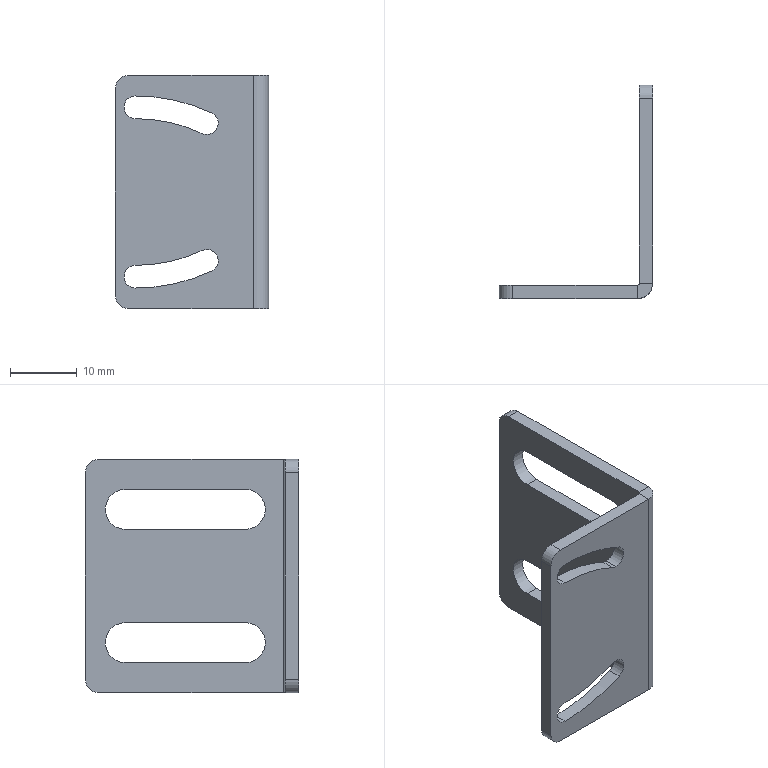Part | SolidWorks | features ICE 2, Fillet 1, FlatPattern 1, HoleWzd 1, MirrorPattern 1, SMBaseFlange 1, SheetMetal 1 | 1 solid | 35 faces | box 23 x 32 x 35 mm | volume 2932 mm3 | cylinder 19 | plane 16 | commonest cylinder face diameters 3.4 x5 4 x4 6 x4 47.4 x2 54.2 x2 0.6 x1
STEP:
#1=CARTESIAN_POINT('',(13.735,0.,26.12));
#2=VERTEX_POINT('',#1);
#3=CARTESIAN_POINT('',(14.453,0.,29.361));
#4=VERTEX_POINT('',#3);
#5=CARTESIAN_POINT('',(13.735,0.,27.82));
#6=DIRECTION('',(0.,-1.,0.));
#7=DIRECTION('',(0.,0.,1.));
#8=AXIS2_PLACEMENT_3D('',#5,#6,#7);
#9=CIRCLE('',#8,1.7);
#10=EDGE_CURVE('',#2,#4,#9,.T.);
#11=ORIENTED_EDGE('',*,*,#10,.F.);
#12=CARTESIAN_POINT('',(13.735,-2.,26.12));
#13=VERTEX_POINT('',#12);
#14=CARTESIAN_POINT('',(13.735,30.,26.12));
#15=DIRECTION('',(0.,-1.,0.));
#16=VECTOR('',#15,1000.);
#17=LINE('',#14,#16);
#18=EDGE_CURVE('',#2,#13,#17,.T.);
#19=ORIENTED_EDGE('',*,*,#18,.T.);
#20=CARTESIAN_POINT('',(14.453,-2.,29.361));
#21=VERTEX_POINT('',#20);
#22=CARTESIAN_POINT('',(13.735,-2.,27.82));
#23=DIRECTION('',(0.,1.,0.));
#24=DIRECTION('',(0.,0.,1.));
#25=AXIS2_PLACEMENT_3D('',#22,#23,#24);
#26=CIRCLE('',#25,1.7);
#27=EDGE_CURVE('',#21,#13,#26,.T.);
#28=ORIENTED_EDGE('',*,*,#27,.F.);
#29=CARTESIAN_POINT('',(14.453,30.,29.361));
#30=DIRECTION('',(0.,-1.,0.));
#31=VECTOR('',#30,1000.);
#32=LINE('',#29,#31);
#33=EDGE_CURVE('',#4,#21,#32,.T.);
#34=ORIENTED_EDGE('',*,*,#33,.F.);
#35=EDGE_LOOP('',(#11,#19,#28,#34));
#36=FACE_OUTER_BOUND('',#35,.T.);
#37=CARTESIAN_POINT('',(13.735,30.,27.82));
#38=DIRECTION('',(0.,-1.,0.));
#39=DIRECTION('',(0.,0.,-1.));
#40=AXIS2_PLACEMENT_3D('',#37,#38,#39);
#41=CYLINDRICAL_SURFACE('',#40,1.7);
#42=ADVANCED_FACE('',(#36),#41,.F.);
#43=CARTESIAN_POINT('',(3.,0.,6.5));
#44=VERTEX_POINT('',#43);
#45=CARTESIAN_POINT('',(13.016,0.,8.721));
#46=VERTEX_POINT('',#45);
#47=CARTESIAN_POINT('',(3.,0.,30.2));
#48=DIRECTION('',(0.,-1.,0.));
#49=DIRECTION('',(0.,0.,1.));
#50=AXIS2_PLACEMENT_3D('',#47,#48,#49);
#51=CIRCLE('',#50,23.7);
#52=EDGE_CURVE('',#44,#46,#51,.T.);
#53=ORIENTED_EDGE('',*,*,#52,.F.);
#54=CARTESIAN_POINT('',(3.,0.,3.1));
#55=VERTEX_POINT('',#54);
#56=CARTESIAN_POINT('',(3.,0.,4.8));
#57=DIRECTION('',(0.,1.,0.));
#58=DIRECTION('',(0.,0.,1.));
#59=AXIS2_PLACEMENT_3D('',#56,#57,#58);
#60=CIRCLE('',#59,1.7);
#61=EDGE_CURVE('',#55,#44,#60,.T.);
#62=ORIENTED_EDGE('',*,*,#61,.F.);
#63=CARTESIAN_POINT('',(14.453,0.,5.639));
#64=VERTEX_POINT('',#63);
#65=CARTESIAN_POINT('',(3.,0.,30.2));
#66=DIRECTION('',(0.,1.,0.));
#67=DIRECTION('',(0.,0.,1.));
#68=AXIS2_PLACEMENT_3D('',#65,#66,#67);
#69=CIRCLE('',#68,27.1);
#70=EDGE_CURVE('',#64,#55,#69,.T.);
#71=ORIENTED_EDGE('',*,*,#70,.F.);
#72=CARTESIAN_POINT('',(13.735,0.,7.18));
#73=DIRECTION('',(0.,1.,0.));
#74=DIRECTION('',(0.,0.,1.));
#75=AXIS2_PLACEMENT_3D('',#72,#73,#74);
#76=CIRCLE('',#75,1.7);
#77=EDGE_CURVE('',#46,#64,#76,.T.);
#78=ORIENTED_EDGE('',*,*,#77,.F.);
#79=EDGE_LOOP('',(#53,#62,#71,#78));
#80=FACE_BOUND('',#79,.T.);
#81=CARTESIAN_POINT('',(0.,0.,33.));
#82=VERTEX_POINT('',#81);
#83=CARTESIAN_POINT('',(0.,0.,2.));
#84=VERTEX_POINT('',#83);
#85=CARTESIAN_POINT('',(0.,0.,35.));
#86=DIRECTION('',(0.,0.,-1.));
#87=VECTOR('',#86,1000.);
#88=LINE('',#85,#87);
#89=EDGE_CURVE('',#82,#84,#88,.T.);
#90=ORIENTED_EDGE('',*,*,#89,.F.);
#91=CARTESIAN_POINT('',(2.,0.,35.));
#92=VERTEX_POINT('',#91);
#93=CARTESIAN_POINT('',(2.,0.,33.));
#94=DIRECTION('',(0.,1.,0.));
#95=DIRECTION('',(0.,0.,1.));
#96=AXIS2_PLACEMENT_3D('',#93,#94,#95);
#97=CIRCLE('',#96,2.);
#98=EDGE_CURVE('',#82,#92,#97,.T.);
#99=ORIENTED_EDGE('',*,*,#98,.T.);
#100=CARTESIAN_POINT('',(20.7,0.,35.));
#101=VERTEX_POINT('',#100);
#102=CARTESIAN_POINT('',(0.,0.,35.));
#103=DIRECTION('',(1.,0.,0.));
#104=VECTOR('',#103,1000.);
#105=LINE('',#102,#104);
#106=EDGE_CURVE('',#92,#101,#105,.T.);
#107=ORIENTED_EDGE('',*,*,#106,.T.);
#108=CARTESIAN_POINT('',(20.7,0.,0.));
#109=VERTEX_POINT('',#108);
#110=CARTESIAN_POINT('',(20.7,0.,35.));
#111=DIRECTION('',(0.,0.,-1.));
#112=VECTOR('',#111,1000.);
#113=LINE('',#110,#112);
#114=EDGE_CURVE('',#101,#109,#113,.T.);
#115=ORIENTED_EDGE('',*,*,#114,.T.);
#116=CARTESIAN_POINT('',(2.,0.,0.));
#117=VERTEX_POINT('',#116);
#118=CARTESIAN_POINT('',(0.,0.,0.));
#119=DIRECTION('',(1.,0.,0.));
#120=VECTOR('',#119,1000.);
#121=LINE('',#118,#120);
#122=EDGE_CURVE('',#117,#109,#121,.T.);
#123=ORIENTED_EDGE('',*,*,#122,.F.);
#124=CARTESIAN_POINT('',(2.,0.,2.));
#125=DIRECTION('',(0.,1.,0.));
#126=DIRECTION('',(0.,0.,1.));
#127=AXIS2_PLACEMENT_3D('',#124,#125,#126);
#128=CIRCLE('',#127,2.);
#129=EDGE_CURVE('',#117,#84,#128,.T.);
#130=ORIENTED_EDGE('',*,*,#129,.T.);
#131=EDGE_LOOP('',(#90,#99,#107,#115,#123,#130));
#132=FACE_OUTER_BOUND('',#131,.T.);
#133=CARTESIAN_POINT('',(13.016,0.,26.279));
#134=VERTEX_POINT('',#133);
#135=CARTESIAN_POINT('',(13.735,0.,27.82));
#136=DIRECTION('',(0.,-1.,0.));
#137=DIRECTION('',(0.,0.,1.));
#138=AXIS2_PLACEMENT_3D('',#135,#136,#137);
#139=CIRCLE('',#138,1.7);
#140=EDGE_CURVE('',#134,#2,#139,.T.);
#141=ORIENTED_EDGE('',*,*,#140,.T.);
#142=ORIENTED_EDGE('',*,*,#10,.T.);
#143=CARTESIAN_POINT('',(3.,0.,31.9));
#144=VERTEX_POINT('',#143);
#145=CARTESIAN_POINT('',(3.,0.,4.8));
#146=DIRECTION('',(0.,-1.,0.));
#147=DIRECTION('',(0.,0.,1.));
#148=AXIS2_PLACEMENT_3D('',#145,#146,#147);
#149=CIRCLE('',#148,27.1);
#150=EDGE_CURVE('',#4,#144,#149,.T.);
#151=ORIENTED_EDGE('',*,*,#150,.T.);
#152=CARTESIAN_POINT('',(3.,0.,28.5));
#153=VERTEX_POINT('',#152);
#154=CARTESIAN_POINT('',(3.,0.,30.2));
#155=DIRECTION('',(0.,1.,0.));
#156=DIRECTION('',(0.,0.,1.));
#157=AXIS2_PLACEMENT_3D('',#154,#155,#156);
#158=CIRCLE('',#157,1.7);
#159=EDGE_CURVE('',#153,#144,#158,.T.);
#160=ORIENTED_EDGE('',*,*,#159,.F.);
#161=CARTESIAN_POINT('',(3.,0.,4.8));
#162=DIRECTION('',(0.,1.,0.));
#163=DIRECTION('',(0.,0.,1.));
#164=AXIS2_PLACEMENT_3D('',#161,#162,#163);
#165=CIRCLE('',#164,23.7);
#166=EDGE_CURVE('',#153,#134,#165,.T.);
#167=ORIENTED_EDGE('',*,*,#166,.T.);
#168=EDGE_LOOP('',(#141,#142,#151,#160,#167));
#169=FACE_BOUND('',#168,.T.);
#170=CARTESIAN_POINT('',(0.,0.,35.));
#171=DIRECTION('',(0.,1.,0.));
#172=DIRECTION('',(0.,0.,1.));
#173=AXIS2_PLACEMENT_3D('',#170,#171,#172);
#174=PLANE('',#173);
#175=ADVANCED_FACE('',(#80,#132,#169),#174,.T.);
#176=CARTESIAN_POINT('',(2.,-2.,35.));
#177=VERTEX_POINT('',#176);
#178=CARTESIAN_POINT('',(20.7,-2.,35.));
#179=VERTEX_POINT('',#178);
#180=CARTESIAN_POINT('',(0.,-2.,35.));
#181=DIRECTION('',(1.,0.,0.));
#182=VECTOR('',#181,1000.);
#183=LINE('',#180,#182);
#184=EDGE_CURVE('',#177,#179,#183,.T.);
#185=ORIENTED_EDGE('',*,*,#184,.F.);
#186=CARTESIAN_POINT('',(0.,-2.,33.));
#187=VERTEX_POINT('',#186);
#188=CARTESIAN_POINT('',(2.,-2.,33.));
#189=DIRECTION('',(0.,-1.,0.));
#190=DIRECTION('',(0.,0.,1.));
#191=AXIS2_PLACEMENT_3D('',#188,#189,#190);
#192=CIRCLE('',#191,2.);
#193=EDGE_CURVE('',#177,#187,#192,.T.);
#194=ORIENTED_EDGE('',*,*,#193,.T.);
#195=CARTESIAN_POINT('',(0.,-2.,2.));
#196=VERTEX_POINT('',#195);
#197=CARTESIAN_POINT('',(0.,-2.,35.));
#198=DIRECTION('',(0.,0.,-1.));
#199=VECTOR('',#198,1000.);
#200=LINE('',#197,#199);
#201=EDGE_CURVE('',#187,#196,#200,.T.);
#202=ORIENTED_EDGE('',*,*,#201,.T.);
#203=CARTESIAN_POINT('',(2.,-2.,0.));
#204=VERTEX_POINT('',#203);
#205=CARTESIAN_POINT('',(2.,-2.,2.));
#206=DIRECTION('',(0.,-1.,0.));
#207=DIRECTION('',(0.,0.,1.));
#208=AXIS2_PLACEMENT_3D('',#205,#206,#207);
#209=CIRCLE('',#208,2.);
#210=EDGE_CURVE('',#196,#204,#209,.T.);
#211=ORIENTED_EDGE('',*,*,#210,.T.);
#212=CARTESIAN_POINT('',(20.7,-2.,0.));
#213=VERTEX_POINT('',#212);
#214=CARTESIAN_POINT('',(0.,-2.,0.));
#215=DIRECTION('',(1.,0.,0.));
#216=VECTOR('',#215,1000.);
#217=LINE('',#214,#216);
#218=EDGE_CURVE('',#204,#213,#217,.T.);
#219=ORIENTED_EDGE('',*,*,#218,.T.);
#220=CARTESIAN_POINT('',(20.7,-2.,35.));
#221=DIRECTION('',(0.,0.,-1.));
#222=VECTOR('',#221,1000.);
#223=LINE('',#220,#222);
#224=EDGE_CURVE('',#179,#213,#223,.T.);
#225=ORIENTED_EDGE('',*,*,#224,.F.);
#226=EDGE_LOOP('',(#185,#194,#202,#211,#219,#225));
#227=FACE_OUTER_BOUND('',#226,.T.);
#228=CARTESIAN_POINT('',(3.,-2.,3.1));
#229=VERTEX_POINT('',#228);
#230=CARTESIAN_POINT('',(3.,-2.,6.5));
#231=VERTEX_POINT('',#230);
#232=CARTESIAN_POINT('',(3.,-2.,4.8));
#233=DIRECTION('',(0.,1.,0.));
#234=DIRECTION('',(0.,0.,1.));
#235=AXIS2_PLACEMENT_3D('',#232,#233,#234);
#236=CIRCLE('',#235,1.7);
#237=EDGE_CURVE('',#229,#231,#236,.T.);
#238=ORIENTED_EDGE('',*,*,#237,.T.);
#239=CARTESIAN_POINT('',(13.016,-2.,8.721));
#240=VERTEX_POINT('',#239);
#241=CARTESIAN_POINT('',(3.,-2.,30.2));
#242=DIRECTION('',(0.,1.,0.));
#243=DIRECTION('',(0.,0.,-1.));
#244=AXIS2_PLACEMENT_3D('',#241,#242,#243);
#245=CIRCLE('',#244,23.7);
#246=EDGE_CURVE('',#240,#231,#245,.T.);
#247=ORIENTED_EDGE('',*,*,#246,.F.);
#248=CARTESIAN_POINT('',(14.453,-2.,5.639));
#249=VERTEX_POINT('',#248);
#250=CARTESIAN_POINT('',(13.735,-2.,7.18));
#251=DIRECTION('',(0.,-1.,0.));
#252=DIRECTION('',(0.,0.,-1.));
#253=AXIS2_PLACEMENT_3D('',#250,#251,#252);
#254=CIRCLE('',#253,1.7);
#255=EDGE_CURVE('',#249,#240,#254,.T.);
#256=ORIENTED_EDGE('',*,*,#255,.F.);
#257=CARTESIAN_POINT('',(3.,-2.,30.2));
#258=DIRECTION('',(0.,-1.,0.));
#259=DIRECTION('',(0.,0.,-1.));
#260=AXIS2_PLACEMENT_3D('',#257,#258,#259);
#261=CIRCLE('',#260,27.1);
#262=EDGE_CURVE('',#229,#249,#261,.T.);
#263=ORIENTED_EDGE('',*,*,#262,.F.);
#264=EDGE_LOOP('',(#238,#247,#256,#263));
#265=FACE_BOUND('',#264,.T.);
#266=CARTESIAN_POINT('',(3.,-2.,31.9));
#267=VERTEX_POINT('',#266);
#268=CARTESIAN_POINT('',(3.,-2.,4.8));
#269=DIRECTION('',(0.,1.,0.));
#270=DIRECTION('',(0.,0.,1.));
#271=AXIS2_PLACEMENT_3D('',#268,#269,#270);
#272=CIRCLE('',#271,27.1);
#273=EDGE_CURVE('',#267,#21,#272,.T.);
#274=ORIENTED_EDGE('',*,*,#273,.T.);
#275=ORIENTED_EDGE('',*,*,#27,.T.);
#276=CARTESIAN_POINT('',(13.016,-2.,26.279));
#277=VERTEX_POINT('',#276);
#278=CARTESIAN_POINT('',(13.735,-2.,27.82));
#279=DIRECTION('',(0.,1.,0.));
#280=DIRECTION('',(0.,0.,1.));
#281=AXIS2_PLACEMENT_3D('',#278,#279,#280);
#282=CIRCLE('',#281,1.7);
#283=EDGE_CURVE('',#13,#277,#282,.T.);
#284=ORIENTED_EDGE('',*,*,#283,.T.);
#285=CARTESIAN_POINT('',(3.,-2.,28.5));
#286=VERTEX_POINT('',#285);
#287=CARTESIAN_POINT('',(3.,-2.,4.8));
#288=DIRECTION('',(0.,-1.,0.));
#289=DIRECTION('',(0.,0.,1.));
#290=AXIS2_PLACEMENT_3D('',#287,#288,#289);
#291=CIRCLE('',#290,23.7);
#292=EDGE_CURVE('',#277,#286,#291,.T.);
#293=ORIENTED_EDGE('',*,*,#292,.T.);
#294=CARTESIAN_POINT('',(3.,-2.,30.2));
#295=DIRECTION('',(0.,1.,0.));
#296=DIRECTION('',(0.,0.,1.));
#297=AXIS2_PLACEMENT_3D('',#294,#295,#296);
#298=CIRCLE('',#297,1.7);
#299=EDGE_CURVE('',#286,#267,#298,.T.);
#300=ORIENTED_EDGE('',*,*,#299,.T.);
#301=EDGE_LOOP('',(#274,#275,#284,#293,#300));
#302=FACE_BOUND('',#301,.T.);
#303=CARTESIAN_POINT('',(0.,-2.,35.));
#304=DIRECTION('',(0.,1.,0.));
#305=DIRECTION('',(0.,0.,1.));
#306=AXIS2_PLACEMENT_3D('',#303,#304,#305);
#307=PLANE('',#306);
#308=ADVANCED_FACE('',(#227,#265,#302),#307,.F.);
#309=CARTESIAN_POINT('',(21.,0.3,35.));
#310=VERTEX_POINT('',#309);
#311=CARTESIAN_POINT('',(23.,0.3,35.));
#312=VERTEX_POINT('',#311);
#313=CARTESIAN_POINT('',(21.,0.3,35.));
#314=DIRECTION('',(1.,0.,0.));
#315=VECTOR('',#314,1000.);
#316=LINE('',#313,#315);
#317=EDGE_CURVE('',#310,#312,#316,.T.);
#318=ORIENTED_EDGE('',*,*,#317,.F.);
#319=CARTESIAN_POINT('',(20.7,0.3,35.));
#320=DIRECTION('',(0.,0.,1.));
#321=DIRECTION('',(-1.,0.,0.));
#322=AXIS2_PLACEMENT_3D('',#319,#320,#321);
#323=CIRCLE('',#322,0.3);
#324=EDGE_CURVE('',#101,#310,#323,.T.);
#325=ORIENTED_EDGE('',*,*,#324,.F.);
#326=CARTESIAN_POINT('',(20.7,-2.,35.));
#327=DIRECTION('',(0.,1.,0.));
#328=VECTOR('',#327,1000.);
#329=LINE('',#326,#328);
#330=EDGE_CURVE('',#179,#101,#329,.T.);
#331=ORIENTED_EDGE('',*,*,#330,.F.);
#332=CARTESIAN_POINT('',(20.7,0.3,35.));
#333=DIRECTION('',(0.,0.,1.));
#334=DIRECTION('',(1.,0.,0.));
#335=AXIS2_PLACEMENT_3D('',#332,#333,#334);
#336=CIRCLE('',#335,2.3);
#337=EDGE_CURVE('',#179,#312,#336,.T.);
#338=ORIENTED_EDGE('',*,*,#337,.T.);
#339=EDGE_LOOP('',(#318,#325,#331,#338));
#340=FACE_OUTER_BOUND('',#339,.T.);
#341=CARTESIAN_POINT('',(21.,0.3,35.));
#342=DIRECTION('',(0.,0.,1.));
#343=DIRECTION('',(1.,0.,0.));
#344=AXIS2_PLACEMENT_3D('',#341,#342,#343);
#345=PLANE('',#344);
#346=ADVANCED_FACE('',(#340),#345,.T.);
#347=CARTESIAN_POINT('',(23.,28.,35.));
#348=VERTEX_POINT('',#347);
#349=CARTESIAN_POINT('',(23.,0.,35.));
#350=DIRECTION('',(0.,1.,0.));
#351=VECTOR('',#350,1000.);
#352=LINE('',#349,#351);
#353=EDGE_CURVE('',#312,#348,#352,.T.);
#354=ORIENTED_EDGE('',*,*,#353,.T.);
#355=CARTESIAN_POINT('',(21.,28.,35.));
#356=VERTEX_POINT('',#355);
#357=CARTESIAN_POINT('',(20.7,28.,35.));
#358=DIRECTION('',(-1.,0.,0.));
#359=VECTOR('',#358,1000.);
#360=LINE('',#357,#359);
#361=EDGE_CURVE('',#348,#356,#360,.T.);
#362=ORIENTED_EDGE('',*,*,#361,.T.);
#363=CARTESIAN_POINT('',(21.,0.,35.));
#364=DIRECTION('',(0.,1.,0.));
#365=VECTOR('',#364,1000.);
#366=LINE('',#363,#365);
#367=EDGE_CURVE('',#310,#356,#366,.T.);
#368=ORIENTED_EDGE('',*,*,#367,.F.);
#369=ORIENTED_EDGE('',*,*,#317,.T.);
#370=EDGE_LOOP('',(#354,#362,#368,#369));
#371=FACE_OUTER_BOUND('',#370,.T.);
#372=CARTESIAN_POINT('',(20.7,-2.,35.));
#373=DIRECTION('',(0.,0.,1.));
#374=DIRECTION('',(1.,0.,0.));
#375=AXIS2_PLACEMENT_3D('',#372,#373,#374);
#376=PLANE('',#375);
#377=ADVANCED_FACE('',(#371),#376,.T.);
#378=CARTESIAN_POINT('',(20.7,0.,0.));
#379=DIRECTION('',(0.,-1.,0.));
#380=VECTOR('',#379,1000.);
#381=LINE('',#378,#380);
#382=EDGE_CURVE('',#109,#213,#381,.T.);
#383=ORIENTED_EDGE('',*,*,#382,.F.);
#384=CARTESIAN_POINT('',(21.,0.3,0.));
#385=VERTEX_POINT('',#384);
#386=CARTESIAN_POINT('',(20.7,0.3,0.));
#387=DIRECTION('',(0.,0.,1.));
#388=DIRECTION('',(-1.,0.,0.));
#389=AXIS2_PLACEMENT_3D('',#386,#387,#388);
#390=CIRCLE('',#389,0.3);
#391=EDGE_CURVE('',#109,#385,#390,.T.);
#392=ORIENTED_EDGE('',*,*,#391,.T.);
#393=CARTESIAN_POINT('',(23.,0.3,0.));
#394=VERTEX_POINT('',#393);
#395=CARTESIAN_POINT('',(23.,0.3,0.));
#396=DIRECTION('',(-1.,0.,0.));
#397=VECTOR('',#396,1000.);
#398=LINE('',#395,#397);
#399=EDGE_CURVE('',#394,#385,#398,.T.);
#400=ORIENTED_EDGE('',*,*,#399,.F.);
#401=CARTESIAN_POINT('',(20.7,0.3,0.));
#402=DIRECTION('',(0.,0.,1.));
#403=DIRECTION('',(1.,0.,0.));
#404=AXIS2_PLACEMENT_3D('',#401,#402,#403);
#405=CIRCLE('',#404,2.3);
#406=EDGE_CURVE('',#213,#394,#405,.T.);
#407=ORIENTED_EDGE('',*,*,#406,.F.);
#408=EDGE_LOOP('',(#383,#392,#400,#407));
#409=FACE_OUTER_BOUND('',#408,.T.);
#410=CARTESIAN_POINT('',(20.7,0.,0.));
#411=DIRECTION('',(0.,0.,-1.));
#412=DIRECTION('',(-1.,0.,0.));
#413=AXIS2_PLACEMENT_3D('',#410,#411,#412);
#414=PLANE('',#413);
#415=ADVANCED_FACE('',(#409),#414,.T.);
#416=ORIENTED_EDGE('',*,*,#218,.F.);
#417=CARTESIAN_POINT('',(2.,0.3,0.));
#418=DIRECTION('',(0.,1.,0.));
#419=VECTOR('',#418,1000.);
#420=LINE('',#417,#419);
#421=EDGE_CURVE('',#204,#117,#420,.T.);
#422=ORIENTED_EDGE('',*,*,#421,.T.);
#423=ORIENTED_EDGE('',*,*,#122,.T.);
#424=ORIENTED_EDGE('',*,*,#382,.T.);
#425=EDGE_LOOP('',(#416,#422,#423,#424));
#426=FACE_OUTER_BOUND('',#425,.T.);
#427=CARTESIAN_POINT('',(23.,0.3,0.));
#428=DIRECTION('',(0.,0.,-1.));
#429=DIRECTION('',(-1.,0.,0.));
#430=AXIS2_PLACEMENT_3D('',#427,#428,#429);
#431=PLANE('',#430);
#432=ADVANCED_FACE('',(#426),#431,.T.);
#433=CARTESIAN_POINT('',(23.,6.,10.5));
#434=VERTEX_POINT('',#433);
#435=CARTESIAN_POINT('',(23.,24.,10.5));
#436=VERTEX_POINT('',#435);
#437=CARTESIAN_POINT('',(23.,24.,10.5));
#438=DIRECTION('',(0.,1.,0.));
#439=VECTOR('',#438,1000.);
#440=LINE('',#437,#439);
#441=EDGE_CURVE('',#434,#436,#440,.T.);
#442=ORIENTED_EDGE('',*,*,#441,.T.);
#443=CARTESIAN_POINT('',(23.,24.,4.5));
#444=VERTEX_POINT('',#443);
#445=CARTESIAN_POINT('',(23.,24.,7.5));
#446=DIRECTION('',(-1.,0.,0.));
#447=DIRECTION('',(0.,0.,1.));
#448=AXIS2_PLACEMENT_3D('',#445,#446,#447);
#449=CIRCLE('',#448,3.);
#450=EDGE_CURVE('',#436,#444,#449,.T.);
#451=ORIENTED_EDGE('',*,*,#450,.T.);
#452=CARTESIAN_POINT('',(23.,6.,4.5));
#453=VERTEX_POINT('',#452);
#454=CARTESIAN_POINT('',(23.,24.,4.5));
#455=DIRECTION('',(0.,-1.,0.));
#456=VECTOR('',#455,1000.);
#457=LINE('',#454,#456);
#458=EDGE_CURVE('',#444,#453,#457,.T.);
#459=ORIENTED_EDGE('',*,*,#458,.T.);
#460=CARTESIAN_POINT('',(23.,6.,7.5));
#461=DIRECTION('',(-1.,0.,0.));
#462=DIRECTION('',(0.,0.,1.));
#463=AXIS2_PLACEMENT_3D('',#460,#461,#462);
#464=CIRCLE('',#463,3.);
#465=EDGE_CURVE('',#453,#434,#464,.T.);
#466=ORIENTED_EDGE('',*,*,#465,.T.);
#467=EDGE_LOOP('',(#442,#451,#459,#466));
#468=FACE_BOUND('',#467,.T.);
#469=CARTESIAN_POINT('',(23.,6.,30.5));
#470=VERTEX_POINT('',#469);
#471=CARTESIAN_POINT('',(23.,24.,30.5));
#472=VERTEX_POINT('',#471);
#473=CARTESIAN_POINT('',(23.,24.,30.5));
#474=DIRECTION('',(0.,1.,0.));
#475=VECTOR('',#474,1000.);
#476=LINE('',#473,#475);
#477=EDGE_CURVE('',#470,#472,#476,.T.);
#478=ORIENTED_EDGE('',*,*,#477,.T.);
#479=CARTESIAN_POINT('',(23.,24.,24.5));
#480=VERTEX_POINT('',#479);
#481=CARTESIAN_POINT('',(23.,24.,27.5));
#482=DIRECTION('',(-1.,0.,0.));
#483=DIRECTION('',(0.,0.,1.));
#484=AXIS2_PLACEMENT_3D('',#481,#482,#483);
#485=CIRCLE('',#484,3.);
#486=EDGE_CURVE('',#472,#480,#485,.T.);
#487=ORIENTED_EDGE('',*,*,#486,.T.);
#488=CARTESIAN_POINT('',(23.,6.,24.5));
#489=VERTEX_POINT('',#488);
#490=CARTESIAN_POINT('',(23.,24.,24.5));
#491=DIRECTION('',(0.,-1.,0.));
#492=VECTOR('',#491,1000.);
#493=LINE('',#490,#492);
#494=EDGE_CURVE('',#480,#489,#493,.T.);
#495=ORIENTED_EDGE('',*,*,#494,.T.);
#496=CARTESIAN_POINT('',(23.,6.,27.5));
#497=DIRECTION('',(-1.,0.,0.));
#498=DIRECTION('',(0.,0.,1.));
#499=AXIS2_PLACEMENT_3D('',#496,#497,#498);
#500=CIRCLE('',#499,3.);
#501=EDGE_CURVE('',#489,#470,#500,.T.);
#502=ORIENTED_EDGE('',*,*,#501,.T.);
#503=EDGE_LOOP('',(#478,#487,#495,#502));
#504=FACE_BOUND('',#503,.T.);
#505=CARTESIAN_POINT('',(23.,28.,0.));
#506=VERTEX_POINT('',#505);
#507=CARTESIAN_POINT('',(23.,0.,0.));
#508=DIRECTION('',(0.,1.,0.));
#509=VECTOR('',#508,1000.);
#510=LINE('',#507,#509);
#511=EDGE_CURVE('',#394,#506,#510,.T.);
#512=ORIENTED_EDGE('',*,*,#511,.T.);
#513=CARTESIAN_POINT('',(23.,30.,2.));
#514=VERTEX_POINT('',#513);
#515=CARTESIAN_POINT('',(23.,28.,2.));
#516=DIRECTION('',(1.,0.,0.));
#517=DIRECTION('',(0.,0.,1.));
#518=AXIS2_PLACEMENT_3D('',#515,#516,#517);
#519=CIRCLE('',#518,2.);
#520=EDGE_CURVE('',#506,#514,#519,.T.);
#521=ORIENTED_EDGE('',*,*,#520,.T.);
#522=CARTESIAN_POINT('',(23.,30.,33.));
#523=VERTEX_POINT('',#522);
#524=CARTESIAN_POINT('',(23.,30.,35.));
#525=DIRECTION('',(0.,0.,-1.));
#526=VECTOR('',#525,1000.);
#527=LINE('',#524,#526);
#528=EDGE_CURVE('',#523,#514,#527,.T.);
#529=ORIENTED_EDGE('',*,*,#528,.F.);
#530=CARTESIAN_POINT('',(23.,28.,33.));
#531=DIRECTION('',(1.,0.,0.));
#532=DIRECTION('',(0.,0.,1.));
#533=AXIS2_PLACEMENT_3D('',#530,#531,#532);
#534=CIRCLE('',#533,2.);
#535=EDGE_CURVE('',#523,#348,#534,.T.);
#536=ORIENTED_EDGE('',*,*,#535,.T.);
#537=ORIENTED_EDGE('',*,*,#353,.F.);
#538=CARTESIAN_POINT('',(23.,0.3,35.));
#539=DIRECTION('',(0.,0.,-1.));
#540=VECTOR('',#539,1000.);
#541=LINE('',#538,#540);
#542=EDGE_CURVE('',#312,#394,#541,.T.);
#543=ORIENTED_EDGE('',*,*,#542,.T.);
#544=EDGE_LOOP('',(#512,#521,#529,#536,#537,#543));
#545=FACE_OUTER_BOUND('',#544,.T.);
#546=CARTESIAN_POINT('',(23.,0.,35.));
#547=DIRECTION('',(-1.,0.,0.));
#548=DIRECTION('',(0.,0.,1.));
#549=AXIS2_PLACEMENT_3D('',#546,#547,#548);
#550=PLANE('',#549);
#551=ADVANCED_FACE('',(#468,#504,#545),#550,.F.);
#552=ORIENTED_EDGE('',*,*,#528,.T.);
#553=CARTESIAN_POINT('',(21.,30.,2.));
#554=VERTEX_POINT('',#553);
#555=CARTESIAN_POINT('',(21.,30.,2.));
#556=DIRECTION('',(-1.,0.,0.));
#557=VECTOR('',#556,1000.);
#558=LINE('',#555,#557);
#559=EDGE_CURVE('',#514,#554,#558,.T.);
#560=ORIENTED_EDGE('',*,*,#559,.T.);
#561=CARTESIAN_POINT('',(21.,30.,33.));
#562=VERTEX_POINT('',#561);
#563=CARTESIAN_POINT('',(21.,30.,35.));
#564=DIRECTION('',(0.,0.,-1.));
#565=VECTOR('',#564,1000.);
#566=LINE('',#563,#565);
#567=EDGE_CURVE('',#562,#554,#566,.T.);
#568=ORIENTED_EDGE('',*,*,#567,.F.);
#569=CARTESIAN_POINT('',(21.,30.,33.));
#570=DIRECTION('',(1.,0.,0.));
#571=VECTOR('',#570,1000.);
#572=LINE('',#569,#571);
#573=EDGE_CURVE('',#562,#523,#572,.T.);
#574=ORIENTED_EDGE('',*,*,#573,.T.);
#575=EDGE_LOOP('',(#552,#560,#568,#574));
#576=FACE_OUTER_BOUND('',#575,.T.);
#577=CARTESIAN_POINT('',(21.,30.,35.));
#578=DIRECTION('',(0.,1.,0.));
#579=DIRECTION('',(0.,0.,1.));
#580=AXIS2_PLACEMENT_3D('',#577,#578,#579);
#581=PLANE('',#580);
#582=ADVANCED_FACE('',(#576),#581,.T.);
#583=CARTESIAN_POINT('',(21.,24.,10.5));
#584=VERTEX_POINT('',#583);
#585=CARTESIAN_POINT('',(21.,24.,4.5));
#586=VERTEX_POINT('',#585);
#587=CARTESIAN_POINT('',(21.,24.,7.5));
#588=DIRECTION('',(-1.,0.,0.));
#589=DIRECTION('',(0.,0.,1.));
#590=AXIS2_PLACEMENT_3D('',#587,#588,#589);
#591=CIRCLE('',#590,3.);
#592=EDGE_CURVE('',#584,#586,#591,.T.);
#593=ORIENTED_EDGE('',*,*,#592,.F.);
#594=CARTESIAN_POINT('',(21.,6.,10.5));
#595=VERTEX_POINT('',#594);
#596=CARTESIAN_POINT('',(21.,24.,10.5));
#597=DIRECTION('',(0.,1.,0.));
#598=VECTOR('',#597,1000.);
#599=LINE('',#596,#598);
#600=EDGE_CURVE('',#595,#584,#599,.T.);
#601=ORIENTED_EDGE('',*,*,#600,.F.);
#602=CARTESIAN_POINT('',(21.,6.,4.5));
#603=VERTEX_POINT('',#602);
#604=CARTESIAN_POINT('',(21.,6.,7.5));
#605=DIRECTION('',(-1.,0.,0.));
#606=DIRECTION('',(0.,0.,1.));
#607=AXIS2_PLACEMENT_3D('',#604,#605,#606);
#608=CIRCLE('',#607,3.);
#609=EDGE_CURVE('',#603,#595,#608,.T.);
#610=ORIENTED_EDGE('',*,*,#609,.F.);
#611=CARTESIAN_POINT('',(21.,24.,4.5));
#612=DIRECTION('',(0.,-1.,0.));
#613=VECTOR('',#612,1000.);
#614=LINE('',#611,#613);
#615=EDGE_CURVE('',#586,#603,#614,.T.);
#616=ORIENTED_EDGE('',*,*,#615,.F.);
#617=EDGE_LOOP('',(#593,#601,#610,#616));
#618=FACE_BOUND('',#617,.T.);
#619=CARTESIAN_POINT('',(21.,24.,30.5));
#620=VERTEX_POINT('',#619);
#621=CARTESIAN_POINT('',(21.,24.,24.5));
#622=VERTEX_POINT('',#621);
#623=CARTESIAN_POINT('',(21.,24.,27.5));
#624=DIRECTION('',(-1.,0.,0.));
#625=DIRECTION('',(0.,0.,1.));
#626=AXIS2_PLACEMENT_3D('',#623,#624,#625);
#627=CIRCLE('',#626,3.);
#628=EDGE_CURVE('',#620,#622,#627,.T.);
#629=ORIENTED_EDGE('',*,*,#628,.F.);
#630=CARTESIAN_POINT('',(21.,6.,30.5));
#631=VERTEX_POINT('',#630);
#632=CARTESIAN_POINT('',(21.,24.,30.5));
#633=DIRECTION('',(0.,1.,0.));
#634=VECTOR('',#633,1000.);
#635=LINE('',#632,#634);
#636=EDGE_CURVE('',#631,#620,#635,.T.);
#637=ORIENTED_EDGE('',*,*,#636,.F.);
#638=CARTESIAN_POINT('',(21.,6.,24.5));
#639=VERTEX_POINT('',#638);
#640=CARTESIAN_POINT('',(21.,6.,27.5));
#641=DIRECTION('',(-1.,0.,0.));
#642=DIRECTION('',(0.,0.,1.));
#643=AXIS2_PLACEMENT_3D('',#640,#641,#642);
#644=CIRCLE('',#643,3.);
#645=EDGE_CURVE('',#639,#631,#644,.T.);
#646=ORIENTED_EDGE('',*,*,#645,.F.);
#647=CARTESIAN_POINT('',(21.,24.,24.5));
#648=DIRECTION('',(0.,-1.,0.));
#649=VECTOR('',#648,1000.);
#650=LINE('',#647,#649);
#651=EDGE_CURVE('',#622,#639,#650,.T.);
#652=ORIENTED_EDGE('',*,*,#651,.F.);
#653=EDGE_LOOP('',(#629,#637,#646,#652));
#654=FACE_BOUND('',#653,.T.);
#655=ORIENTED_EDGE('',*,*,#567,.T.);
#656=CARTESIAN_POINT('',(21.,28.,0.));
#657=VERTEX_POINT('',#656);
#658=CARTESIAN_POINT('',(21.,28.,2.));
#659=DIRECTION('',(-1.,0.,0.));
#660=DIRECTION('',(0.,0.,1.));
#661=AXIS2_PLACEMENT_3D('',#658,#659,#660);
#662=CIRCLE('',#661,2.);
#663=EDGE_CURVE('',#554,#657,#662,.T.);
#664=ORIENTED_EDGE('',*,*,#663,.T.);
#665=CARTESIAN_POINT('',(21.,0.,0.));
#666=DIRECTION('',(0.,1.,0.));
#667=VECTOR('',#666,1000.);
#668=LINE('',#665,#667);
#669=EDGE_CURVE('',#385,#657,#668,.T.);
#670=ORIENTED_EDGE('',*,*,#669,.F.);
#671=CARTESIAN_POINT('',(21.,0.3,35.));
#672=DIRECTION('',(0.,0.,-1.));
#673=VECTOR('',#672,1000.);
#674=LINE('',#671,#673);
#675=EDGE_CURVE('',#310,#385,#674,.T.);
#676=ORIENTED_EDGE('',*,*,#675,.F.);
#677=ORIENTED_EDGE('',*,*,#367,.T.);
#678=CARTESIAN_POINT('',(21.,28.,33.));
#679=DIRECTION('',(-1.,0.,0.));
#680=DIRECTION('',(0.,0.,1.));
#681=AXIS2_PLACEMENT_3D('',#678,#679,#680);
#682=CIRCLE('',#681,2.);
#683=EDGE_CURVE('',#356,#562,#682,.T.);
#684=ORIENTED_EDGE('',*,*,#683,.T.);
#685=EDGE_LOOP('',(#655,#664,#670,#676,#677,#684));
#686=FACE_OUTER_BOUND('',#685,.T.);
#687=CARTESIAN_POINT('',(21.,0.,35.));
#688=DIRECTION('',(-1.,0.,0.));
#689=DIRECTION('',(0.,0.,1.));
#690=AXIS2_PLACEMENT_3D('',#687,#688,#689);
#691=PLANE('',#690);
#692=ADVANCED_FACE('',(#618,#654,#686),#691,.T.);
#693=ORIENTED_EDGE('',*,*,#391,.F.);
#694=ORIENTED_EDGE('',*,*,#114,.F.);
#695=ORIENTED_EDGE('',*,*,#324,.T.);
#696=ORIENTED_EDGE('',*,*,#675,.T.);
#697=EDGE_LOOP('',(#693,#694,#695,#696));
#698=FACE_OUTER_BOUND('',#697,.T.);
#699=CARTESIAN_POINT('',(20.7,0.3,35.));
#700=DIRECTION('',(0.,0.,-1.));
#701=DIRECTION('',(-1.,0.,0.));
#702=AXIS2_PLACEMENT_3D('',#699,#700,#701);
#703=CYLINDRICAL_SURFACE('',#702,0.3);
#704=ADVANCED_FACE('',(#698),#703,.F.);
#705=ORIENTED_EDGE('',*,*,#201,.F.);
#706=CARTESIAN_POINT('',(0.,0.,33.));
#707=DIRECTION('',(0.,1.,0.));
#708=VECTOR('',#707,1000.);
#709=LINE('',#706,#708);
#710=EDGE_CURVE('',#187,#82,#709,.T.);
#711=ORIENTED_EDGE('',*,*,#710,.T.);
#712=ORIENTED_EDGE('',*,*,#89,.T.);
#713=CARTESIAN_POINT('',(0.,-2.,2.));
#714=DIRECTION('',(0.,-1.,0.));
#715=VECTOR('',#714,1000.);
#716=LINE('',#713,#715);
#717=EDGE_CURVE('',#84,#196,#716,.T.);
#718=ORIENTED_EDGE('',*,*,#717,.T.);
#719=EDGE_LOOP('',(#705,#711,#712,#718));
#720=FACE_OUTER_BOUND('',#719,.T.);
#721=CARTESIAN_POINT('',(0.,-2.,35.));
#722=DIRECTION('',(-1.,0.,0.));
#723=DIRECTION('',(0.,0.,1.));
#724=AXIS2_PLACEMENT_3D('',#721,#722,#723);
#725=PLANE('',#724);
#726=ADVANCED_FACE('',(#720),#725,.T.);
#727=ORIENTED_EDGE('',*,*,#406,.T.);
#728=ORIENTED_EDGE('',*,*,#542,.F.);
#729=ORIENTED_EDGE('',*,*,#337,.F.);
#730=ORIENTED_EDGE('',*,*,#224,.T.);
#731=EDGE_LOOP('',(#727,#728,#729,#730));
#732=FACE_OUTER_BOUND('',#731,.T.);
#733=CARTESIAN_POINT('',(20.7,0.3,35.));
#734=DIRECTION('',(0.,0.,-1.));
#735=DIRECTION('',(-1.,0.,0.));
#736=AXIS2_PLACEMENT_3D('',#733,#734,#735);
#737=CYLINDRICAL_SURFACE('',#736,2.3);
#738=ADVANCED_FACE('',(#732),#737,.T.);
#739=ORIENTED_EDGE('',*,*,#106,.F.);
#740=CARTESIAN_POINT('',(2.,-2.,35.));
#741=DIRECTION('',(0.,-1.,0.));
#742=VECTOR('',#741,1000.);
#743=LINE('',#740,#742);
#744=EDGE_CURVE('',#92,#177,#743,.T.);
#745=ORIENTED_EDGE('',*,*,#744,.T.);
#746=ORIENTED_EDGE('',*,*,#184,.T.);
#747=ORIENTED_EDGE('',*,*,#330,.T.);
#748=EDGE_LOOP('',(#739,#745,#746,#747));
#749=FACE_OUTER_BOUND('',#748,.T.);
#750=CARTESIAN_POINT('',(20.7,0.3,35.));
#751=DIRECTION('',(0.,0.,-1.));
#752=DIRECTION('',(-1.,0.,0.));
#753=AXIS2_PLACEMENT_3D('',#750,#751,#752);
#754=PLANE('',#753);
#755=ADVANCED_FACE('',(#749),#754,.F.);
#756=ORIENTED_EDGE('',*,*,#669,.T.);
#757=CARTESIAN_POINT('',(20.7,28.,0.));
#758=DIRECTION('',(1.,0.,0.));
#759=VECTOR('',#758,1000.);
#760=LINE('',#757,#759);
#761=EDGE_CURVE('',#657,#506,#760,.T.);
#762=ORIENTED_EDGE('',*,*,#761,.T.);
#763=ORIENTED_EDGE('',*,*,#511,.F.);
#764=ORIENTED_EDGE('',*,*,#399,.T.);
#765=EDGE_LOOP('',(#756,#762,#763,#764));
#766=FACE_OUTER_BOUND('',#765,.T.);
#767=CARTESIAN_POINT('',(20.7,0.3,0.));
#768=DIRECTION('',(0.,0.,-1.));
#769=DIRECTION('',(-1.,0.,0.));
#770=AXIS2_PLACEMENT_3D('',#767,#768,#769);
#771=PLANE('',#770);
#772=ADVANCED_FACE('',(#766),#771,.T.);
#773=ORIENTED_EDGE('',*,*,#159,.T.);
#774=CARTESIAN_POINT('',(3.,14.,31.9));
#775=DIRECTION('',(0.,-1.,0.));
#776=VECTOR('',#775,1000.);
#777=LINE('',#774,#776);
#778=EDGE_CURVE('',#144,#267,#777,.T.);
#779=ORIENTED_EDGE('',*,*,#778,.T.);
#780=ORIENTED_EDGE('',*,*,#299,.F.);
#781=CARTESIAN_POINT('',(3.,14.,28.5));
#782=DIRECTION('',(0.,-1.,0.));
#783=VECTOR('',#782,1000.);
#784=LINE('',#781,#783);
#785=EDGE_CURVE('',#153,#286,#784,.T.);
#786=ORIENTED_EDGE('',*,*,#785,.F.);
#787=EDGE_LOOP('',(#773,#779,#780,#786));
#788=FACE_OUTER_BOUND('',#787,.T.);
#789=CARTESIAN_POINT('',(3.,0.,30.2));
#790=DIRECTION('',(0.,1.,0.));
#791=DIRECTION('',(0.,0.,1.));
#792=AXIS2_PLACEMENT_3D('',#789,#790,#791);
#793=CYLINDRICAL_SURFACE('',#792,1.7);
#794=ADVANCED_FACE('',(#788),#793,.F.);
#795=ORIENTED_EDGE('',*,*,#61,.T.);
#796=CARTESIAN_POINT('',(3.,14.,6.5));
#797=DIRECTION('',(0.,-1.,0.));
#798=VECTOR('',#797,1000.);
#799=LINE('',#796,#798);
#800=EDGE_CURVE('',#44,#231,#799,.T.);
#801=ORIENTED_EDGE('',*,*,#800,.T.);
#802=ORIENTED_EDGE('',*,*,#237,.F.);
#803=CARTESIAN_POINT('',(3.,14.,3.1));
#804=DIRECTION('',(0.,-1.,0.));
#805=VECTOR('',#804,1000.);
#806=LINE('',#803,#805);
#807=EDGE_CURVE('',#55,#229,#806,.T.);
#808=ORIENTED_EDGE('',*,*,#807,.F.);
#809=EDGE_LOOP('',(#795,#801,#802,#808));
#810=FACE_OUTER_BOUND('',#809,.T.);
#811=CARTESIAN_POINT('',(3.,0.,4.8));
#812=DIRECTION('',(0.,1.,0.));
#813=DIRECTION('',(0.,0.,1.));
#814=AXIS2_PLACEMENT_3D('',#811,#812,#813);
#815=CYLINDRICAL_SURFACE('',#814,1.7);
#816=ADVANCED_FACE('',(#810),#815,.F.);
#817=ORIENTED_EDGE('',*,*,#52,.T.);
#818=CARTESIAN_POINT('',(13.016,30.,8.721));
#819=DIRECTION('',(0.,-1.,0.));
#820=VECTOR('',#819,1000.);
#821=LINE('',#818,#820);
#822=EDGE_CURVE('',#46,#240,#821,.T.);
#823=ORIENTED_EDGE('',*,*,#822,.T.);
#824=ORIENTED_EDGE('',*,*,#246,.T.);
#825=ORIENTED_EDGE('',*,*,#800,.F.);
#826=EDGE_LOOP('',(#817,#823,#824,#825));
#827=FACE_OUTER_BOUND('',#826,.T.);
#828=CARTESIAN_POINT('',(3.,30.,30.2));
#829=DIRECTION('',(0.,-1.,0.));
#830=DIRECTION('',(0.,0.,-1.));
#831=AXIS2_PLACEMENT_3D('',#828,#829,#830);
#832=CYLINDRICAL_SURFACE('',#831,23.7);
#833=ADVANCED_FACE('',(#827),#832,.T.);
#834=ORIENTED_EDGE('',*,*,#77,.T.);
#835=CARTESIAN_POINT('',(14.453,30.,5.639));
#836=DIRECTION('',(0.,-1.,0.));
#837=VECTOR('',#836,1000.);
#838=LINE('',#835,#837);
#839=EDGE_CURVE('',#64,#249,#838,.T.);
#840=ORIENTED_EDGE('',*,*,#839,.T.);
#841=ORIENTED_EDGE('',*,*,#255,.T.);
#842=ORIENTED_EDGE('',*,*,#822,.F.);
#843=EDGE_LOOP('',(#834,#840,#841,#842));
#844=FACE_OUTER_BOUND('',#843,.T.);
#845=CARTESIAN_POINT('',(13.735,30.,7.18));
#846=DIRECTION('',(0.,-1.,0.));
#847=DIRECTION('',(0.,0.,-1.));
#848=AXIS2_PLACEMENT_3D('',#845,#846,#847);
#849=CYLINDRICAL_SURFACE('',#848,1.7);
#850=ADVANCED_FACE('',(#844),#849,.F.);
#851=ORIENTED_EDGE('',*,*,#70,.T.);
#852=ORIENTED_EDGE('',*,*,#807,.T.);
#853=ORIENTED_EDGE('',*,*,#262,.T.);
#854=ORIENTED_EDGE('',*,*,#839,.F.);
#855=EDGE_LOOP('',(#851,#852,#853,#854));
#856=FACE_OUTER_BOUND('',#855,.T.);
#857=CARTESIAN_POINT('',(3.,30.,30.2));
#858=DIRECTION('',(0.,-1.,0.));
#859=DIRECTION('',(0.,0.,-1.));
#860=AXIS2_PLACEMENT_3D('',#857,#858,#859);
#861=CYLINDRICAL_SURFACE('',#860,27.1);
#862=ADVANCED_FACE('',(#856),#861,.F.);
#863=ORIENTED_EDGE('',*,*,#663,.F.);
#864=ORIENTED_EDGE('',*,*,#559,.F.);
#865=ORIENTED_EDGE('',*,*,#520,.F.);
#866=ORIENTED_EDGE('',*,*,#761,.F.);
#867=EDGE_LOOP('',(#863,#864,#865,#866));
#868=FACE_OUTER_BOUND('',#867,.T.);
#869=CARTESIAN_POINT('',(20.7,28.,2.));
#870=DIRECTION('',(1.,0.,0.));
#871=DIRECTION('',(0.,0.,-1.));
#872=AXIS2_PLACEMENT_3D('',#869,#870,#871);
#873=CYLINDRICAL_SURFACE('',#872,2.);
#874=ADVANCED_FACE('',(#868),#873,.T.);
#875=ORIENTED_EDGE('',*,*,#683,.F.);
#876=ORIENTED_EDGE('',*,*,#361,.F.);
#877=ORIENTED_EDGE('',*,*,#535,.F.);
#878=ORIENTED_EDGE('',*,*,#573,.F.);
#879=EDGE_LOOP('',(#875,#876,#877,#878));
#880=FACE_OUTER_BOUND('',#879,.T.);
#881=CARTESIAN_POINT('',(21.,28.,33.));
#882=DIRECTION('',(1.,0.,0.));
#883=DIRECTION('',(0.,0.,-1.));
#884=AXIS2_PLACEMENT_3D('',#881,#882,#883);
#885=CYLINDRICAL_SURFACE('',#884,2.);
#886=ADVANCED_FACE('',(#880),#885,.T.);
#887=ORIENTED_EDGE('',*,*,#193,.F.);
#888=ORIENTED_EDGE('',*,*,#744,.F.);
#889=ORIENTED_EDGE('',*,*,#98,.F.);
#890=ORIENTED_EDGE('',*,*,#710,.F.);
#891=EDGE_LOOP('',(#887,#888,#889,#890));
#892=FACE_OUTER_BOUND('',#891,.T.);
#893=CARTESIAN_POINT('',(2.,-2.,33.));
#894=DIRECTION('',(0.,-1.,0.));
#895=DIRECTION('',(0.,0.,-1.));
#896=AXIS2_PLACEMENT_3D('',#893,#894,#895);
#897=CYLINDRICAL_SURFACE('',#896,2.);
#898=ADVANCED_FACE('',(#892),#897,.T.);
#899=ORIENTED_EDGE('',*,*,#210,.F.);
#900=ORIENTED_EDGE('',*,*,#717,.F.);
#901=ORIENTED_EDGE('',*,*,#129,.F.);
#902=ORIENTED_EDGE('',*,*,#421,.F.);
#903=EDGE_LOOP('',(#899,#900,#901,#902));
#904=FACE_OUTER_BOUND('',#903,.T.);
#905=CARTESIAN_POINT('',(2.,0.3,2.));
#906=DIRECTION('',(0.,1.,0.));
#907=DIRECTION('',(0.,0.,1.));
#908=AXIS2_PLACEMENT_3D('',#905,#906,#907);
#909=CYLINDRICAL_SURFACE('',#908,2.);
#910=ADVANCED_FACE('',(#904),#909,.T.);
#911=ORIENTED_EDGE('',*,*,#628,.T.);
#912=CARTESIAN_POINT('',(23.,24.,24.5));
#913=DIRECTION('',(-1.,0.,0.));
#914=VECTOR('',#913,1000.);
#915=LINE('',#912,#914);
#916=EDGE_CURVE('',#480,#622,#915,.T.);
#917=ORIENTED_EDGE('',*,*,#916,.F.);
#918=ORIENTED_EDGE('',*,*,#486,.F.);
#919=CARTESIAN_POINT('',(23.,24.,30.5));
#920=DIRECTION('',(-1.,0.,0.));
#921=VECTOR('',#920,1000.);
#922=LINE('',#919,#921);
#923=EDGE_CURVE('',#472,#620,#922,.T.);
#924=ORIENTED_EDGE('',*,*,#923,.T.);
#925=EDGE_LOOP('',(#911,#917,#918,#924));
#926=FACE_OUTER_BOUND('',#925,.T.);
#927=CARTESIAN_POINT('',(23.,24.,27.5));
#928=DIRECTION('',(-1.,0.,0.));
#929=DIRECTION('',(0.,0.,1.));
#930=AXIS2_PLACEMENT_3D('',#927,#928,#929);
#931=CYLINDRICAL_SURFACE('',#930,3.);
#932=ADVANCED_FACE('',(#926),#931,.F.);
#933=ORIENTED_EDGE('',*,*,#636,.T.);
#934=ORIENTED_EDGE('',*,*,#923,.F.);
#935=ORIENTED_EDGE('',*,*,#477,.F.);
#936=CARTESIAN_POINT('',(23.,6.,30.5));
#937=DIRECTION('',(-1.,0.,0.));
#938=VECTOR('',#937,1000.);
#939=LINE('',#936,#938);
#940=EDGE_CURVE('',#470,#631,#939,.T.);
#941=ORIENTED_EDGE('',*,*,#940,.T.);
#942=EDGE_LOOP('',(#933,#934,#935,#941));
#943=FACE_OUTER_BOUND('',#942,.T.);
#944=CARTESIAN_POINT('',(23.,24.,30.5));
#945=DIRECTION('',(0.,0.,1.));
#946=DIRECTION('',(0.,-1.,0.));
#947=AXIS2_PLACEMENT_3D('',#944,#945,#946);
#948=PLANE('',#947);
#949=ADVANCED_FACE('',(#943),#948,.F.);
#950=ORIENTED_EDGE('',*,*,#645,.T.);
#951=ORIENTED_EDGE('',*,*,#940,.F.);
#952=ORIENTED_EDGE('',*,*,#501,.F.);
#953=CARTESIAN_POINT('',(23.,6.,24.5));
#954=DIRECTION('',(-1.,0.,0.));
#955=VECTOR('',#954,1000.);
#956=LINE('',#953,#955);
#957=EDGE_CURVE('',#489,#639,#956,.T.);
#958=ORIENTED_EDGE('',*,*,#957,.T.);
#959=EDGE_LOOP('',(#950,#951,#952,#958));
#960=FACE_OUTER_BOUND('',#959,.T.);
#961=CARTESIAN_POINT('',(23.,6.,27.5));
#962=DIRECTION('',(-1.,0.,0.));
#963=DIRECTION('',(0.,0.,1.));
#964=AXIS2_PLACEMENT_3D('',#961,#962,#963);
#965=CYLINDRICAL_SURFACE('',#964,3.);
#966=ADVANCED_FACE('',(#960),#965,.F.);
#967=ORIENTED_EDGE('',*,*,#651,.T.);
#968=ORIENTED_EDGE('',*,*,#957,.F.);
#969=ORIENTED_EDGE('',*,*,#494,.F.);
#970=ORIENTED_EDGE('',*,*,#916,.T.);
#971=EDGE_LOOP('',(#967,#968,#969,#970));
#972=FACE_OUTER_BOUND('',#971,.T.);
#973=CARTESIAN_POINT('',(23.,24.,24.5));
#974=DIRECTION('',(0.,0.,-1.));
#975=DIRECTION('',(0.,1.,0.));
#976=AXIS2_PLACEMENT_3D('',#973,#974,#975);
#977=PLANE('',#976);
#978=ADVANCED_FACE('',(#972),#977,.F.);
#979=ORIENTED_EDGE('',*,*,#592,.T.);
#980=CARTESIAN_POINT('',(23.,24.,4.5));
#981=DIRECTION('',(-1.,0.,0.));
#982=VECTOR('',#981,1000.);
#983=LINE('',#980,#982);
#984=EDGE_CURVE('',#444,#586,#983,.T.);
#985=ORIENTED_EDGE('',*,*,#984,.F.);
#986=ORIENTED_EDGE('',*,*,#450,.F.);
#987=CARTESIAN_POINT('',(23.,24.,10.5));
#988=DIRECTION('',(-1.,0.,0.));
#989=VECTOR('',#988,1000.);
#990=LINE('',#987,#989);
#991=EDGE_CURVE('',#436,#584,#990,.T.);
#992=ORIENTED_EDGE('',*,*,#991,.T.);
#993=EDGE_LOOP('',(#979,#985,#986,#992));
#994=FACE_OUTER_BOUND('',#993,.T.);
#995=CARTESIAN_POINT('',(23.,24.,7.5));
#996=DIRECTION('',(-1.,0.,0.));
#997=DIRECTION('',(0.,0.,1.));
#998=AXIS2_PLACEMENT_3D('',#995,#996,#997);
#999=CYLINDRICAL_SURFACE('',#998,3.);
#1000=ADVANCED_FACE('',(#994),#999,.F.);
#1001=ORIENTED_EDGE('',*,*,#600,.T.);
#1002=ORIENTED_EDGE('',*,*,#991,.F.);
#1003=ORIENTED_EDGE('',*,*,#441,.F.);
#1004=CARTESIAN_POINT('',(23.,6.,10.5));
#1005=DIRECTION('',(-1.,0.,0.));
#1006=VECTOR('',#1005,1000.);
#1007=LINE('',#1004,#1006);
#1008=EDGE_CURVE('',#434,#595,#1007,.T.);
#1009=ORIENTED_EDGE('',*,*,#1008,.T.);
#1010=EDGE_LOOP('',(#1001,#1002,#1003,#1009));
#1011=FACE_OUTER_BOUND('',#1010,.T.);
#1012=CARTESIAN_POINT('',(23.,24.,10.5));
#1013=DIRECTION('',(0.,0.,1.));
#1014=DIRECTION('',(0.,-1.,0.));
#1015=AXIS2_PLACEMENT_3D('',#1012,#1013,#1014);
#1016=PLANE('',#1015);
#1017=ADVANCED_FACE('',(#1011),#1016,.F.);
#1018=ORIENTED_EDGE('',*,*,#609,.T.);
#1019=ORIENTED_EDGE('',*,*,#1008,.F.);
#1020=ORIENTED_EDGE('',*,*,#465,.F.);
#1021=CARTESIAN_POINT('',(23.,6.,4.5));
#1022=DIRECTION('',(-1.,0.,0.));
#1023=VECTOR('',#1022,1000.);
#1024=LINE('',#1021,#1023);
#1025=EDGE_CURVE('',#453,#603,#1024,.T.);
#1026=ORIENTED_EDGE('',*,*,#1025,.T.);
#1027=EDGE_LOOP('',(#1018,#1019,#1020,#1026));
#1028=FACE_OUTER_BOUND('',#1027,.T.);
#1029=CARTESIAN_POINT('',(23.,6.,7.5));
#1030=DIRECTION('',(-1.,0.,0.));
#1031=DIRECTION('',(0.,0.,1.));
#1032=AXIS2_PLACEMENT_3D('',#1029,#1030,#1031);
#1033=CYLINDRICAL_SURFACE('',#1032,3.);
#1034=ADVANCED_FACE('',(#1028),#1033,.F.);
#1035=ORIENTED_EDGE('',*,*,#615,.T.);
#1036=ORIENTED_EDGE('',*,*,#1025,.F.);
#1037=ORIENTED_EDGE('',*,*,#458,.F.);
#1038=ORIENTED_EDGE('',*,*,#984,.T.);
#1039=EDGE_LOOP('',(#1035,#1036,#1037,#1038));
#1040=FACE_OUTER_BOUND('',#1039,.T.);
#1041=CARTESIAN_POINT('',(23.,24.,4.5));
#1042=DIRECTION('',(0.,0.,-1.));
#1043=DIRECTION('',(0.,1.,0.));
#1044=AXIS2_PLACEMENT_3D('',#1041,#1042,#1043);
#1045=PLANE('',#1044);
#1046=ADVANCED_FACE('',(#1040),#1045,.F.);
#1047=ORIENTED_EDGE('',*,*,#33,.T.);
#1048=ORIENTED_EDGE('',*,*,#273,.F.);
#1049=ORIENTED_EDGE('',*,*,#778,.F.);
#1050=ORIENTED_EDGE('',*,*,#150,.F.);
#1051=EDGE_LOOP('',(#1047,#1048,#1049,#1050));
#1052=FACE_OUTER_BOUND('',#1051,.T.);
#1053=CARTESIAN_POINT('',(3.,30.,4.8));
#1054=DIRECTION('',(0.,-1.,0.));
#1055=DIRECTION('',(0.,0.,-1.));
#1056=AXIS2_PLACEMENT_3D('',#1053,#1054,#1055);
#1057=CYLINDRICAL_SURFACE('',#1056,27.1);
#1058=ADVANCED_FACE('',(#1052),#1057,.F.);
#1059=ORIENTED_EDGE('',*,*,#18,.F.);
#1060=ORIENTED_EDGE('',*,*,#140,.F.);
#1061=CARTESIAN_POINT('',(13.016,30.,26.279));
#1062=DIRECTION('',(0.,-1.,0.));
#1063=VECTOR('',#1062,1000.);
#1064=LINE('',#1061,#1063);
#1065=EDGE_CURVE('',#134,#277,#1064,.T.);
#1066=ORIENTED_EDGE('',*,*,#1065,.T.);
#1067=ORIENTED_EDGE('',*,*,#283,.F.);
#1068=EDGE_LOOP('',(#1059,#1060,#1066,#1067));
#1069=FACE_OUTER_BOUND('',#1068,.T.);
#1070=CARTESIAN_POINT('',(13.735,30.,27.82));
#1071=DIRECTION('',(0.,-1.,0.));
#1072=DIRECTION('',(0.,0.,-1.));
#1073=AXIS2_PLACEMENT_3D('',#1070,#1071,#1072);
#1074=CYLINDRICAL_SURFACE('',#1073,1.7);
#1075=ADVANCED_FACE('',(#1069),#1074,.F.);
#1076=ORIENTED_EDGE('',*,*,#785,.T.);
#1077=ORIENTED_EDGE('',*,*,#292,.F.);
#1078=ORIENTED_EDGE('',*,*,#1065,.F.);
#1079=ORIENTED_EDGE('',*,*,#166,.F.);
#1080=EDGE_LOOP('',(#1076,#1077,#1078,#1079));
#1081=FACE_OUTER_BOUND('',#1080,.T.);
#1082=CARTESIAN_POINT('',(3.,30.,4.8));
#1083=DIRECTION('',(0.,-1.,0.));
#1084=DIRECTION('',(0.,0.,-1.));
#1085=AXIS2_PLACEMENT_3D('',#1082,#1083,#1084);
#1086=CYLINDRICAL_SURFACE('',#1085,23.7);
#1087=ADVANCED_FACE('',(#1081),#1086,.T.);
#1088=CLOSED_SHELL('',(#42,#175,#308,#346,#377,#415,#432,#551,#582,#692,#704,#726,#738,#755,#772,#794,#816,#833,#850,#862,#874,#886,#898,#910,#932,#949,#966,#978,#1000,#1017,#1034,#1046,#1058,#1075,#1087));
#1089=MANIFOLD_SOLID_BREP('',#1088);
#1090=CARTESIAN_POINT('',(0.,0.,0.));
#1091=DIRECTION('',(0.,0.,1.));
#1092=DIRECTION('',(1.,0.,0.));
#1093=AXIS2_PLACEMENT_3D('',#1090,#1091,#1092);
#1094=(LENGTH_UNIT()NAMED_UNIT(*)SI_UNIT(.MILLI.,.METRE.));
#1095=UNCERTAINTY_MEASURE_WITH_UNIT(LENGTH_MEASURE(0.00001),#1094,'','');
#1096=(NAMED_UNIT(*)PLANE_ANGLE_UNIT()SI_UNIT($,.RADIAN.));
#1097=(NAMED_UNIT(*)SI_UNIT($,.STERADIAN.)SOLID_ANGLE_UNIT());
#1098=(GEOMETRIC_REPRESENTATION_CONTEXT(3)GLOBAL_UNCERTAINTY_ASSIGNED_CONTEXT((#1095))GLOBAL_UNIT_ASSIGNED_CONTEXT((#1094,#1096,#1097))REPRESENTATION_CONTEXT('',''));
#1099=ADVANCED_BREP_SHAPE_REPRESENTATION('',(#1089,#1093),#1098);